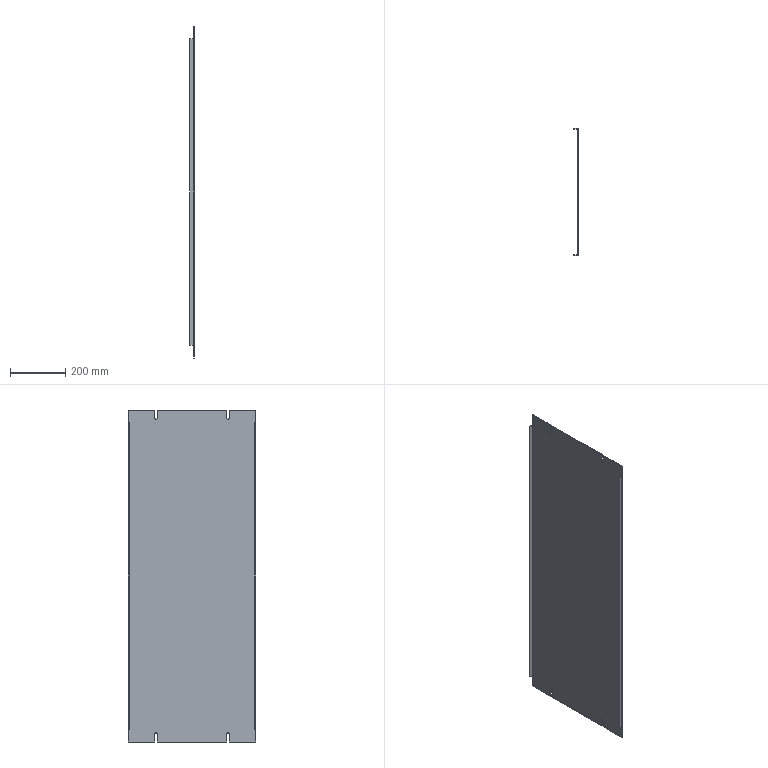Part | STEP file | Electrical board | 1 solid | 48 faces | box 15 x 460 x 1200 mm | volume 1154703 mm3 | plane 38 | cylinder 10 | commonest cylinder face diameters 8 x6 3 x2 7 x2
STEP:
#1=CARTESIAN_POINT('',(2.,-126.,-570.));
#2=VERTEX_POINT('',#1);
#3=CARTESIAN_POINT('',(2.,-130.,-566.));
#4=VERTEX_POINT('',#3);
#5=CARTESIAN_POINT('',(2.,-130.,-570.));
#6=DIRECTION('',(1.,0.,0.));
#7=DIRECTION('',(0.,0.,1.));
#8=AXIS2_PLACEMENT_3D('',#5,#6,#7);
#9=CIRCLE('',#8,4.);
#10=EDGE_CURVE('',#2,#4,#9,.T.);
#11=ORIENTED_EDGE('',*,*,#10,.T.);
#12=CARTESIAN_POINT('',(0.,-130.,-566.));
#13=VERTEX_POINT('',#12);
#14=CARTESIAN_POINT('',(2.,-130.,-566.));
#15=DIRECTION('',(-1.,0.,0.));
#16=VECTOR('',#15,1000.);
#17=LINE('',#14,#16);
#18=EDGE_CURVE('',#4,#13,#17,.T.);
#19=ORIENTED_EDGE('',*,*,#18,.T.);
#20=CARTESIAN_POINT('',(0.,-126.,-570.));
#21=VERTEX_POINT('',#20);
#22=CARTESIAN_POINT('',(0.,-130.,-570.));
#23=DIRECTION('',(1.,0.,0.));
#24=DIRECTION('',(0.,0.,1.));
#25=AXIS2_PLACEMENT_3D('',#22,#23,#24);
#26=CIRCLE('',#25,4.);
#27=EDGE_CURVE('',#21,#13,#26,.T.);
#28=ORIENTED_EDGE('',*,*,#27,.F.);
#29=CARTESIAN_POINT('',(2.,-126.,-570.));
#30=DIRECTION('',(-1.,0.,0.));
#31=VECTOR('',#30,1000.);
#32=LINE('',#29,#31);
#33=EDGE_CURVE('',#2,#21,#32,.T.);
#34=ORIENTED_EDGE('',*,*,#33,.F.);
#35=EDGE_LOOP('',(#11,#19,#28,#34));
#36=FACE_OUTER_BOUND('',#35,.T.);
#37=CARTESIAN_POINT('',(2.,-130.,-570.));
#38=DIRECTION('',(-1.,0.,0.));
#39=DIRECTION('',(0.,0.,1.));
#40=AXIS2_PLACEMENT_3D('',#37,#38,#39);
#41=CYLINDRICAL_SURFACE('',#40,4.);
#42=ADVANCED_FACE('',(#36),#41,.F.);
#43=CARTESIAN_POINT('',(2.,134.,-570.));
#44=VERTEX_POINT('',#43);
#45=CARTESIAN_POINT('',(2.,130.,-566.));
#46=VERTEX_POINT('',#45);
#47=CARTESIAN_POINT('',(2.,130.,-570.));
#48=DIRECTION('',(1.,0.,0.));
#49=DIRECTION('',(0.,0.,1.));
#50=AXIS2_PLACEMENT_3D('',#47,#48,#49);
#51=CIRCLE('',#50,4.);
#52=EDGE_CURVE('',#44,#46,#51,.T.);
#53=ORIENTED_EDGE('',*,*,#52,.T.);
#54=CARTESIAN_POINT('',(0.,130.,-566.));
#55=VERTEX_POINT('',#54);
#56=CARTESIAN_POINT('',(2.,130.,-566.));
#57=DIRECTION('',(-1.,0.,0.));
#58=VECTOR('',#57,1000.);
#59=LINE('',#56,#58);
#60=EDGE_CURVE('',#46,#55,#59,.T.);
#61=ORIENTED_EDGE('',*,*,#60,.T.);
#62=CARTESIAN_POINT('',(0.,134.,-570.));
#63=VERTEX_POINT('',#62);
#64=CARTESIAN_POINT('',(0.,130.,-570.));
#65=DIRECTION('',(1.,0.,0.));
#66=DIRECTION('',(0.,0.,1.));
#67=AXIS2_PLACEMENT_3D('',#64,#65,#66);
#68=CIRCLE('',#67,4.);
#69=EDGE_CURVE('',#63,#55,#68,.T.);
#70=ORIENTED_EDGE('',*,*,#69,.F.);
#71=CARTESIAN_POINT('',(2.,134.,-570.));
#72=DIRECTION('',(-1.,0.,0.));
#73=VECTOR('',#72,1000.);
#74=LINE('',#71,#73);
#75=EDGE_CURVE('',#44,#63,#74,.T.);
#76=ORIENTED_EDGE('',*,*,#75,.F.);
#77=EDGE_LOOP('',(#53,#61,#70,#76));
#78=FACE_OUTER_BOUND('',#77,.T.);
#79=CARTESIAN_POINT('',(2.,130.,-570.));
#80=DIRECTION('',(-1.,0.,0.));
#81=DIRECTION('',(0.,0.,1.));
#82=AXIS2_PLACEMENT_3D('',#79,#80,#81);
#83=CYLINDRICAL_SURFACE('',#82,4.);
#84=ADVANCED_FACE('',(#78),#83,.F.);
#85=CARTESIAN_POINT('',(2.,-225.5,554.));
#86=VERTEX_POINT('',#85);
#87=CARTESIAN_POINT('',(2.,-225.5,555.));
#88=VERTEX_POINT('',#87);
#89=CARTESIAN_POINT('',(2.,-225.5,555.));
#90=DIRECTION('',(0.,0.,1.));
#91=VECTOR('',#90,1000.);
#92=LINE('',#89,#91);
#93=EDGE_CURVE('',#86,#88,#92,.T.);
#94=ORIENTED_EDGE('',*,*,#93,.F.);
#95=CARTESIAN_POINT('',(2.,-226.5,554.));
#96=VERTEX_POINT('',#95);
#97=CARTESIAN_POINT('',(2.,-225.5,554.));
#98=DIRECTION('',(0.,1.,0.));
#99=VECTOR('',#98,1000.);
#100=LINE('',#97,#99);
#101=EDGE_CURVE('',#96,#86,#100,.T.);
#102=ORIENTED_EDGE('',*,*,#101,.F.);
#103=CARTESIAN_POINT('',(2.,-226.5,-554.));
#104=VERTEX_POINT('',#103);
#105=CARTESIAN_POINT('',(2.,-226.5,0.));
#106=DIRECTION('',(0.,0.,1.));
#107=VECTOR('',#106,1000.);
#108=LINE('',#105,#107);
#109=EDGE_CURVE('',#104,#96,#108,.T.);
#110=ORIENTED_EDGE('',*,*,#109,.F.);
#111=CARTESIAN_POINT('',(2.,-225.5,-554.));
#112=VERTEX_POINT('',#111);
#113=CARTESIAN_POINT('',(2.,-226.5,-554.));
#114=DIRECTION('',(0.,-1.,0.));
#115=VECTOR('',#114,1000.);
#116=LINE('',#113,#115);
#117=EDGE_CURVE('',#112,#104,#116,.T.);
#118=ORIENTED_EDGE('',*,*,#117,.F.);
#119=CARTESIAN_POINT('',(2.,-225.5,-555.));
#120=VERTEX_POINT('',#119);
#121=CARTESIAN_POINT('',(2.,-225.5,-554.));
#122=DIRECTION('',(0.,0.,1.));
#123=VECTOR('',#122,1000.);
#124=LINE('',#121,#123);
#125=EDGE_CURVE('',#120,#112,#124,.T.);
#126=ORIENTED_EDGE('',*,*,#125,.F.);
#127=CARTESIAN_POINT('',(2.,-230.,-555.));
#128=VERTEX_POINT('',#127);
#129=CARTESIAN_POINT('',(2.,0.,-555.));
#130=DIRECTION('',(0.,1.,0.));
#131=VECTOR('',#130,1000.);
#132=LINE('',#129,#131);
#133=EDGE_CURVE('',#128,#120,#132,.T.);
#134=ORIENTED_EDGE('',*,*,#133,.F.);
#135=CARTESIAN_POINT('',(2.,-230.,-600.));
#136=VERTEX_POINT('',#135);
#137=CARTESIAN_POINT('',(2.,-230.,0.));
#138=DIRECTION('',(0.,0.,1.));
#139=VECTOR('',#138,1000.);
#140=LINE('',#137,#139);
#141=EDGE_CURVE('',#136,#128,#140,.T.);
#142=ORIENTED_EDGE('',*,*,#141,.F.);
#143=CARTESIAN_POINT('',(2.,-134.,-600.));
#144=VERTEX_POINT('',#143);
#145=CARTESIAN_POINT('',(2.,0.,-600.));
#146=DIRECTION('',(0.,-1.,0.));
#147=VECTOR('',#146,1000.);
#148=LINE('',#145,#147);
#149=EDGE_CURVE('',#144,#136,#148,.T.);
#150=ORIENTED_EDGE('',*,*,#149,.F.);
#151=CARTESIAN_POINT('',(2.,-134.,-570.));
#152=VERTEX_POINT('',#151);
#153=CARTESIAN_POINT('',(2.,-134.,0.));
#154=DIRECTION('',(0.,0.,-1.));
#155=VECTOR('',#154,1000.);
#156=LINE('',#153,#155);
#157=EDGE_CURVE('',#152,#144,#156,.T.);
#158=ORIENTED_EDGE('',*,*,#157,.F.);
#159=CARTESIAN_POINT('',(2.,-130.,-570.));
#160=DIRECTION('',(1.,0.,0.));
#161=DIRECTION('',(0.,0.,1.));
#162=AXIS2_PLACEMENT_3D('',#159,#160,#161);
#163=CIRCLE('',#162,4.);
#164=EDGE_CURVE('',#4,#152,#163,.T.);
#165=ORIENTED_EDGE('',*,*,#164,.F.);
#166=ORIENTED_EDGE('',*,*,#10,.F.);
#167=CARTESIAN_POINT('',(2.,-126.,-600.));
#168=VERTEX_POINT('',#167);
#169=CARTESIAN_POINT('',(2.,-126.,0.));
#170=DIRECTION('',(0.,0.,1.));
#171=VECTOR('',#170,1000.);
#172=LINE('',#169,#171);
#173=EDGE_CURVE('',#168,#2,#172,.T.);
#174=ORIENTED_EDGE('',*,*,#173,.F.);
#175=CARTESIAN_POINT('',(2.,126.,-600.));
#176=VERTEX_POINT('',#175);
#177=CARTESIAN_POINT('',(2.,0.,-600.));
#178=DIRECTION('',(0.,-1.,0.));
#179=VECTOR('',#178,1000.);
#180=LINE('',#177,#179);
#181=EDGE_CURVE('',#176,#168,#180,.T.);
#182=ORIENTED_EDGE('',*,*,#181,.F.);
#183=CARTESIAN_POINT('',(2.,126.,-570.));
#184=VERTEX_POINT('',#183);
#185=CARTESIAN_POINT('',(2.,126.,0.));
#186=DIRECTION('',(0.,0.,-1.));
#187=VECTOR('',#186,1000.);
#188=LINE('',#185,#187);
#189=EDGE_CURVE('',#184,#176,#188,.T.);
#190=ORIENTED_EDGE('',*,*,#189,.F.);
#191=CARTESIAN_POINT('',(2.,130.,-570.));
#192=DIRECTION('',(1.,0.,0.));
#193=DIRECTION('',(0.,0.,1.));
#194=AXIS2_PLACEMENT_3D('',#191,#192,#193);
#195=CIRCLE('',#194,4.);
#196=EDGE_CURVE('',#46,#184,#195,.T.);
#197=ORIENTED_EDGE('',*,*,#196,.F.);
#198=ORIENTED_EDGE('',*,*,#52,.F.);
#199=CARTESIAN_POINT('',(2.,134.,-600.));
#200=VERTEX_POINT('',#199);
#201=CARTESIAN_POINT('',(2.,134.,0.));
#202=DIRECTION('',(0.,0.,1.));
#203=VECTOR('',#202,1000.);
#204=LINE('',#201,#203);
#205=EDGE_CURVE('',#200,#44,#204,.T.);
#206=ORIENTED_EDGE('',*,*,#205,.F.);
#207=CARTESIAN_POINT('',(2.,230.,-600.));
#208=VERTEX_POINT('',#207);
#209=CARTESIAN_POINT('',(2.,0.,-600.));
#210=DIRECTION('',(0.,-1.,0.));
#211=VECTOR('',#210,1000.);
#212=LINE('',#209,#211);
#213=EDGE_CURVE('',#208,#200,#212,.T.);
#214=ORIENTED_EDGE('',*,*,#213,.F.);
#215=CARTESIAN_POINT('',(2.,230.,-555.));
#216=VERTEX_POINT('',#215);
#217=CARTESIAN_POINT('',(2.,230.,0.));
#218=DIRECTION('',(0.,0.,-1.));
#219=VECTOR('',#218,1000.);
#220=LINE('',#217,#219);
#221=EDGE_CURVE('',#216,#208,#220,.T.);
#222=ORIENTED_EDGE('',*,*,#221,.F.);
#223=CARTESIAN_POINT('',(2.,225.5,-555.));
#224=VERTEX_POINT('',#223);
#225=CARTESIAN_POINT('',(2.,0.,-555.));
#226=DIRECTION('',(0.,1.,0.));
#227=VECTOR('',#226,1000.);
#228=LINE('',#225,#227);
#229=EDGE_CURVE('',#224,#216,#228,.T.);
#230=ORIENTED_EDGE('',*,*,#229,.F.);
#231=CARTESIAN_POINT('',(2.,225.5,-554.));
#232=VERTEX_POINT('',#231);
#233=CARTESIAN_POINT('',(2.,225.5,-555.));
#234=DIRECTION('',(0.,0.,-1.));
#235=VECTOR('',#234,1000.);
#236=LINE('',#233,#235);
#237=EDGE_CURVE('',#232,#224,#236,.T.);
#238=ORIENTED_EDGE('',*,*,#237,.F.);
#239=CARTESIAN_POINT('',(2.,226.5,-554.));
#240=VERTEX_POINT('',#239);
#241=CARTESIAN_POINT('',(2.,225.5,-554.));
#242=DIRECTION('',(0.,-1.,0.));
#243=VECTOR('',#242,1000.);
#244=LINE('',#241,#243);
#245=EDGE_CURVE('',#240,#232,#244,.T.);
#246=ORIENTED_EDGE('',*,*,#245,.F.);
#247=CARTESIAN_POINT('',(2.,226.5,554.));
#248=VERTEX_POINT('',#247);
#249=CARTESIAN_POINT('',(2.,226.5,0.));
#250=DIRECTION('',(0.,0.,-1.));
#251=VECTOR('',#250,1000.);
#252=LINE('',#249,#251);
#253=EDGE_CURVE('',#248,#240,#252,.T.);
#254=ORIENTED_EDGE('',*,*,#253,.F.);
#255=CARTESIAN_POINT('',(2.,225.5,554.));
#256=VERTEX_POINT('',#255);
#257=CARTESIAN_POINT('',(2.,226.5,554.));
#258=DIRECTION('',(0.,1.,0.));
#259=VECTOR('',#258,1000.);
#260=LINE('',#257,#259);
#261=EDGE_CURVE('',#256,#248,#260,.T.);
#262=ORIENTED_EDGE('',*,*,#261,.F.);
#263=CARTESIAN_POINT('',(2.,225.5,555.));
#264=VERTEX_POINT('',#263);
#265=CARTESIAN_POINT('',(2.,225.5,554.));
#266=DIRECTION('',(0.,0.,-1.));
#267=VECTOR('',#266,1000.);
#268=LINE('',#265,#267);
#269=EDGE_CURVE('',#264,#256,#268,.T.);
#270=ORIENTED_EDGE('',*,*,#269,.F.);
#271=CARTESIAN_POINT('',(2.,230.,555.));
#272=VERTEX_POINT('',#271);
#273=CARTESIAN_POINT('',(2.,0.,555.));
#274=DIRECTION('',(0.,-1.,0.));
#275=VECTOR('',#274,1000.);
#276=LINE('',#273,#275);
#277=EDGE_CURVE('',#272,#264,#276,.T.);
#278=ORIENTED_EDGE('',*,*,#277,.F.);
#279=CARTESIAN_POINT('',(2.,230.,600.));
#280=VERTEX_POINT('',#279);
#281=CARTESIAN_POINT('',(2.,230.,0.));
#282=DIRECTION('',(0.,0.,-1.));
#283=VECTOR('',#282,1000.);
#284=LINE('',#281,#283);
#285=EDGE_CURVE('',#280,#272,#284,.T.);
#286=ORIENTED_EDGE('',*,*,#285,.F.);
#287=CARTESIAN_POINT('',(2.,134.,600.));
#288=VERTEX_POINT('',#287);
#289=CARTESIAN_POINT('',(2.,0.,600.));
#290=DIRECTION('',(0.,1.,0.));
#291=VECTOR('',#290,1000.);
#292=LINE('',#289,#291);
#293=EDGE_CURVE('',#288,#280,#292,.T.);
#294=ORIENTED_EDGE('',*,*,#293,.F.);
#295=CARTESIAN_POINT('',(2.,134.,570.));
#296=VERTEX_POINT('',#295);
#297=CARTESIAN_POINT('',(2.,134.,0.));
#298=DIRECTION('',(0.,0.,1.));
#299=VECTOR('',#298,1000.);
#300=LINE('',#297,#299);
#301=EDGE_CURVE('',#296,#288,#300,.T.);
#302=ORIENTED_EDGE('',*,*,#301,.F.);
#303=CARTESIAN_POINT('',(2.,126.,570.));
#304=VERTEX_POINT('',#303);
#305=CARTESIAN_POINT('',(2.,130.,570.));
#306=DIRECTION('',(1.,0.,0.));
#307=DIRECTION('',(0.,0.,1.));
#308=AXIS2_PLACEMENT_3D('',#305,#306,#307);
#309=CIRCLE('',#308,4.);
#310=EDGE_CURVE('',#304,#296,#309,.T.);
#311=ORIENTED_EDGE('',*,*,#310,.F.);
#312=CARTESIAN_POINT('',(2.,126.,600.));
#313=VERTEX_POINT('',#312);
#314=CARTESIAN_POINT('',(2.,126.,0.));
#315=DIRECTION('',(0.,0.,-1.));
#316=VECTOR('',#315,1000.);
#317=LINE('',#314,#316);
#318=EDGE_CURVE('',#313,#304,#317,.T.);
#319=ORIENTED_EDGE('',*,*,#318,.F.);
#320=CARTESIAN_POINT('',(2.,-126.,600.));
#321=VERTEX_POINT('',#320);
#322=CARTESIAN_POINT('',(2.,0.,600.));
#323=DIRECTION('',(0.,1.,0.));
#324=VECTOR('',#323,1000.);
#325=LINE('',#322,#324);
#326=EDGE_CURVE('',#321,#313,#325,.T.);
#327=ORIENTED_EDGE('',*,*,#326,.F.);
#328=CARTESIAN_POINT('',(2.,-126.,570.));
#329=VERTEX_POINT('',#328);
#330=CARTESIAN_POINT('',(2.,-126.,0.));
#331=DIRECTION('',(0.,0.,1.));
#332=VECTOR('',#331,1000.);
#333=LINE('',#330,#332);
#334=EDGE_CURVE('',#329,#321,#333,.T.);
#335=ORIENTED_EDGE('',*,*,#334,.F.);
#336=CARTESIAN_POINT('',(2.,-134.,570.));
#337=VERTEX_POINT('',#336);
#338=CARTESIAN_POINT('',(2.,-130.,570.));
#339=DIRECTION('',(1.,0.,0.));
#340=DIRECTION('',(0.,0.,1.));
#341=AXIS2_PLACEMENT_3D('',#338,#339,#340);
#342=CIRCLE('',#341,4.);
#343=EDGE_CURVE('',#337,#329,#342,.T.);
#344=ORIENTED_EDGE('',*,*,#343,.F.);
#345=CARTESIAN_POINT('',(2.,-134.,600.));
#346=VERTEX_POINT('',#345);
#347=CARTESIAN_POINT('',(2.,-134.,0.));
#348=DIRECTION('',(0.,0.,-1.));
#349=VECTOR('',#348,1000.);
#350=LINE('',#347,#349);
#351=EDGE_CURVE('',#346,#337,#350,.T.);
#352=ORIENTED_EDGE('',*,*,#351,.F.);
#353=CARTESIAN_POINT('',(2.,-230.,600.));
#354=VERTEX_POINT('',#353);
#355=CARTESIAN_POINT('',(2.,0.,600.));
#356=DIRECTION('',(0.,1.,0.));
#357=VECTOR('',#356,1000.);
#358=LINE('',#355,#357);
#359=EDGE_CURVE('',#354,#346,#358,.T.);
#360=ORIENTED_EDGE('',*,*,#359,.F.);
#361=CARTESIAN_POINT('',(2.,-230.,555.));
#362=VERTEX_POINT('',#361);
#363=CARTESIAN_POINT('',(2.,-230.,0.));
#364=DIRECTION('',(0.,0.,1.));
#365=VECTOR('',#364,1000.);
#366=LINE('',#363,#365);
#367=EDGE_CURVE('',#362,#354,#366,.T.);
#368=ORIENTED_EDGE('',*,*,#367,.F.);
#369=CARTESIAN_POINT('',(2.,0.,555.));
#370=DIRECTION('',(0.,-1.,0.));
#371=VECTOR('',#370,1000.);
#372=LINE('',#369,#371);
#373=EDGE_CURVE('',#88,#362,#372,.T.);
#374=ORIENTED_EDGE('',*,*,#373,.F.);
#375=EDGE_LOOP('',(#94,#102,#110,#118,#126,#134,#142,#150,#158,#165,#166,#174,#182,#190,#197,#198,#206,#214,#222,#230,#238,#246,#254,#262,#270,#278,#286,#294,#302,#311,#319,#327,#335,#344,#352,#360,#368,#374));
#376=FACE_OUTER_BOUND('',#375,.T.);
#377=CARTESIAN_POINT('',(2.,0.,0.));
#378=DIRECTION('',(-1.,0.,0.));
#379=DIRECTION('',(0.,0.,1.));
#380=AXIS2_PLACEMENT_3D('',#377,#378,#379);
#381=PLANE('',#380);
#382=ADVANCED_FACE('',(#376),#381,.F.);
#383=CARTESIAN_POINT('',(0.,-225.5,555.));
#384=VERTEX_POINT('',#383);
#385=CARTESIAN_POINT('',(0.,-230.,555.));
#386=VERTEX_POINT('',#385);
#387=CARTESIAN_POINT('',(0.,-232.,555.));
#388=DIRECTION('',(0.,-1.,0.));
#389=VECTOR('',#388,1000.);
#390=LINE('',#387,#389);
#391=EDGE_CURVE('',#384,#386,#390,.T.);
#392=ORIENTED_EDGE('',*,*,#391,.F.);
#393=CARTESIAN_POINT('',(2.,-225.5,555.));
#394=DIRECTION('',(-1.,0.,0.));
#395=VECTOR('',#394,1000.);
#396=LINE('',#393,#395);
#397=EDGE_CURVE('',#88,#384,#396,.T.);
#398=ORIENTED_EDGE('',*,*,#397,.F.);
#399=ORIENTED_EDGE('',*,*,#373,.T.);
#400=CARTESIAN_POINT('',(2.,-230.,555.));
#401=DIRECTION('',(1.,0.,0.));
#402=VECTOR('',#401,1000.);
#403=LINE('',#400,#402);
#404=EDGE_CURVE('',#386,#362,#403,.T.);
#405=ORIENTED_EDGE('',*,*,#404,.F.);
#406=EDGE_LOOP('',(#392,#398,#399,#405));
#407=FACE_OUTER_BOUND('',#406,.T.);
#408=CARTESIAN_POINT('',(2.,-232.,555.));
#409=DIRECTION('',(0.,0.,1.));
#410=DIRECTION('',(1.,0.,0.));
#411=AXIS2_PLACEMENT_3D('',#408,#409,#410);
#412=PLANE('',#411);
#413=ADVANCED_FACE('',(#407),#412,.F.);
#414=CARTESIAN_POINT('',(-1.5,-230.,554.));
#415=VERTEX_POINT('',#414);
#416=CARTESIAN_POINT('',(-1.5,-230.,-554.));
#417=VERTEX_POINT('',#416);
#418=CARTESIAN_POINT('',(-1.5,-230.,554.));
#419=DIRECTION('',(0.,0.,-1.));
#420=VECTOR('',#419,1000.);
#421=LINE('',#418,#420);
#422=EDGE_CURVE('',#415,#417,#421,.T.);
#423=ORIENTED_EDGE('',*,*,#422,.T.);
#424=CARTESIAN_POINT('',(-1.5,-226.5,-554.));
#425=DIRECTION('',(0.,0.,1.));
#426=DIRECTION('',(1.,0.,0.));
#427=AXIS2_PLACEMENT_3D('',#424,#425,#426);
#428=CIRCLE('',#427,3.5);
#429=EDGE_CURVE('',#417,#104,#428,.T.);
#430=ORIENTED_EDGE('',*,*,#429,.T.);
#431=ORIENTED_EDGE('',*,*,#109,.T.);
#432=CARTESIAN_POINT('',(-1.5,-226.5,554.));
#433=DIRECTION('',(0.,0.,-1.));
#434=DIRECTION('',(1.,0.,0.));
#435=AXIS2_PLACEMENT_3D('',#432,#433,#434);
#436=CIRCLE('',#435,3.5);
#437=EDGE_CURVE('',#96,#415,#436,.T.);
#438=ORIENTED_EDGE('',*,*,#437,.T.);
#439=EDGE_LOOP('',(#423,#430,#431,#438));
#440=FACE_OUTER_BOUND('',#439,.T.);
#441=CARTESIAN_POINT('',(-1.5,-226.5,554.));
#442=DIRECTION('',(0.,0.,1.));
#443=DIRECTION('',(1.,0.,0.));
#444=AXIS2_PLACEMENT_3D('',#441,#442,#443);
#445=CYLINDRICAL_SURFACE('',#444,3.5);
#446=ADVANCED_FACE('',(#440),#445,.T.);
#447=CARTESIAN_POINT('',(0.,-225.5,-555.));
#448=VERTEX_POINT('',#447);
#449=CARTESIAN_POINT('',(0.,-230.,-555.));
#450=VERTEX_POINT('',#449);
#451=CARTESIAN_POINT('',(0.,-232.,-555.));
#452=DIRECTION('',(0.,-1.,0.));
#453=VECTOR('',#452,1000.);
#454=LINE('',#451,#453);
#455=EDGE_CURVE('',#448,#450,#454,.T.);
#456=ORIENTED_EDGE('',*,*,#455,.T.);
#457=CARTESIAN_POINT('',(2.,-230.,-555.));
#458=DIRECTION('',(1.,0.,0.));
#459=VECTOR('',#458,1000.);
#460=LINE('',#457,#459);
#461=EDGE_CURVE('',#450,#128,#460,.T.);
#462=ORIENTED_EDGE('',*,*,#461,.T.);
#463=ORIENTED_EDGE('',*,*,#133,.T.);
#464=CARTESIAN_POINT('',(2.,-225.5,-555.));
#465=DIRECTION('',(-1.,0.,0.));
#466=VECTOR('',#465,1000.);
#467=LINE('',#464,#466);
#468=EDGE_CURVE('',#120,#448,#467,.T.);
#469=ORIENTED_EDGE('',*,*,#468,.T.);
#470=EDGE_LOOP('',(#456,#462,#463,#469));
#471=FACE_OUTER_BOUND('',#470,.T.);
#472=CARTESIAN_POINT('',(2.,-232.,-555.));
#473=DIRECTION('',(0.,0.,1.));
#474=DIRECTION('',(1.,0.,0.));
#475=AXIS2_PLACEMENT_3D('',#472,#473,#474);
#476=PLANE('',#475);
#477=ADVANCED_FACE('',(#471),#476,.T.);
#478=CARTESIAN_POINT('',(0.,-230.,-600.));
#479=VERTEX_POINT('',#478);
#480=CARTESIAN_POINT('',(0.,-230.,600.));
#481=DIRECTION('',(0.,0.,1.));
#482=VECTOR('',#481,1000.);
#483=LINE('',#480,#482);
#484=EDGE_CURVE('',#479,#450,#483,.T.);
#485=ORIENTED_EDGE('',*,*,#484,.F.);
#486=CARTESIAN_POINT('',(2.,-230.,-600.));
#487=DIRECTION('',(-1.,0.,0.));
#488=VECTOR('',#487,1000.);
#489=LINE('',#486,#488);
#490=EDGE_CURVE('',#136,#479,#489,.T.);
#491=ORIENTED_EDGE('',*,*,#490,.F.);
#492=ORIENTED_EDGE('',*,*,#141,.T.);
#493=ORIENTED_EDGE('',*,*,#461,.F.);
#494=EDGE_LOOP('',(#485,#491,#492,#493));
#495=FACE_OUTER_BOUND('',#494,.T.);
#496=CARTESIAN_POINT('',(2.,-230.,600.));
#497=DIRECTION('',(0.,1.,0.));
#498=DIRECTION('',(0.,0.,1.));
#499=AXIS2_PLACEMENT_3D('',#496,#497,#498);
#500=PLANE('',#499);
#501=ADVANCED_FACE('',(#495),#500,.F.);
#502=CARTESIAN_POINT('',(0.,-134.,-600.));
#503=VERTEX_POINT('',#502);
#504=CARTESIAN_POINT('',(0.,-230.,-600.));
#505=DIRECTION('',(0.,-1.,0.));
#506=VECTOR('',#505,1000.);
#507=LINE('',#504,#506);
#508=EDGE_CURVE('',#503,#479,#507,.T.);
#509=ORIENTED_EDGE('',*,*,#508,.F.);
#510=CARTESIAN_POINT('',(2.,-134.,-600.));
#511=DIRECTION('',(-1.,0.,0.));
#512=VECTOR('',#511,1000.);
#513=LINE('',#510,#512);
#514=EDGE_CURVE('',#144,#503,#513,.T.);
#515=ORIENTED_EDGE('',*,*,#514,.F.);
#516=ORIENTED_EDGE('',*,*,#149,.T.);
#517=ORIENTED_EDGE('',*,*,#490,.T.);
#518=EDGE_LOOP('',(#509,#515,#516,#517));
#519=FACE_OUTER_BOUND('',#518,.T.);
#520=CARTESIAN_POINT('',(2.,-230.,-600.));
#521=DIRECTION('',(0.,0.,1.));
#522=DIRECTION('',(1.,0.,0.));
#523=AXIS2_PLACEMENT_3D('',#520,#521,#522);
#524=PLANE('',#523);
#525=ADVANCED_FACE('',(#519),#524,.F.);
#526=CARTESIAN_POINT('',(0.,-134.,-570.));
#527=VERTEX_POINT('',#526);
#528=CARTESIAN_POINT('',(0.,-134.,-630.));
#529=DIRECTION('',(0.,0.,-1.));
#530=VECTOR('',#529,1000.);
#531=LINE('',#528,#530);
#532=EDGE_CURVE('',#527,#503,#531,.T.);
#533=ORIENTED_EDGE('',*,*,#532,.F.);
#534=CARTESIAN_POINT('',(2.,-134.,-570.));
#535=DIRECTION('',(-1.,0.,0.));
#536=VECTOR('',#535,1000.);
#537=LINE('',#534,#536);
#538=EDGE_CURVE('',#152,#527,#537,.T.);
#539=ORIENTED_EDGE('',*,*,#538,.F.);
#540=ORIENTED_EDGE('',*,*,#157,.T.);
#541=ORIENTED_EDGE('',*,*,#514,.T.);
#542=EDGE_LOOP('',(#533,#539,#540,#541));
#543=FACE_OUTER_BOUND('',#542,.T.);
#544=CARTESIAN_POINT('',(2.,-134.,-630.));
#545=DIRECTION('',(0.,-1.,0.));
#546=DIRECTION('',(0.,0.,-1.));
#547=AXIS2_PLACEMENT_3D('',#544,#545,#546);
#548=PLANE('',#547);
#549=ADVANCED_FACE('',(#543),#548,.F.);
#550=ORIENTED_EDGE('',*,*,#18,.F.);
#551=ORIENTED_EDGE('',*,*,#164,.T.);
#552=ORIENTED_EDGE('',*,*,#538,.T.);
#553=CARTESIAN_POINT('',(0.,-130.,-570.));
#554=DIRECTION('',(1.,0.,0.));
#555=DIRECTION('',(0.,0.,1.));
#556=AXIS2_PLACEMENT_3D('',#553,#554,#555);
#557=CIRCLE('',#556,4.);
#558=EDGE_CURVE('',#13,#527,#557,.T.);
#559=ORIENTED_EDGE('',*,*,#558,.F.);
#560=EDGE_LOOP('',(#550,#551,#552,#559));
#561=FACE_OUTER_BOUND('',#560,.T.);
#562=CARTESIAN_POINT('',(2.,-130.,-570.));
#563=DIRECTION('',(-1.,0.,0.));
#564=DIRECTION('',(0.,0.,1.));
#565=AXIS2_PLACEMENT_3D('',#562,#563,#564);
#566=CYLINDRICAL_SURFACE('',#565,4.);
#567=ADVANCED_FACE('',(#561),#566,.F.);
#568=CARTESIAN_POINT('',(0.,-126.,-600.));
#569=VERTEX_POINT('',#568);
#570=CARTESIAN_POINT('',(0.,-126.,-630.));
#571=DIRECTION('',(0.,0.,1.));
#572=VECTOR('',#571,1000.);
#573=LINE('',#570,#572);
#574=EDGE_CURVE('',#569,#21,#573,.T.);
#575=ORIENTED_EDGE('',*,*,#574,.F.);
#576=CARTESIAN_POINT('',(2.,-126.,-600.));
#577=DIRECTION('',(-1.,0.,0.));
#578=VECTOR('',#577,1000.);
#579=LINE('',#576,#578);
#580=EDGE_CURVE('',#168,#569,#579,.T.);
#581=ORIENTED_EDGE('',*,*,#580,.F.);
#582=ORIENTED_EDGE('',*,*,#173,.T.);
#583=ORIENTED_EDGE('',*,*,#33,.T.);
#584=EDGE_LOOP('',(#575,#581,#582,#583));
#585=FACE_OUTER_BOUND('',#584,.T.);
#586=CARTESIAN_POINT('',(2.,-126.,-630.));
#587=DIRECTION('',(0.,1.,0.));
#588=DIRECTION('',(0.,0.,1.));
#589=AXIS2_PLACEMENT_3D('',#586,#587,#588);
#590=PLANE('',#589);
#591=ADVANCED_FACE('',(#585),#590,.F.);
#592=CARTESIAN_POINT('',(0.,126.,-600.));
#593=VERTEX_POINT('',#592);
#594=CARTESIAN_POINT('',(0.,-230.,-600.));
#595=DIRECTION('',(0.,-1.,0.));
#596=VECTOR('',#595,1000.);
#597=LINE('',#594,#596);
#598=EDGE_CURVE('',#593,#569,#597,.T.);
#599=ORIENTED_EDGE('',*,*,#598,.F.);
#600=CARTESIAN_POINT('',(2.,126.,-600.));
#601=DIRECTION('',(-1.,0.,0.));
#602=VECTOR('',#601,1000.);
#603=LINE('',#600,#602);
#604=EDGE_CURVE('',#176,#593,#603,.T.);
#605=ORIENTED_EDGE('',*,*,#604,.F.);
#606=ORIENTED_EDGE('',*,*,#181,.T.);
#607=ORIENTED_EDGE('',*,*,#580,.T.);
#608=EDGE_LOOP('',(#599,#605,#606,#607));
#609=FACE_OUTER_BOUND('',#608,.T.);
#610=CARTESIAN_POINT('',(2.,-230.,-600.));
#611=DIRECTION('',(0.,0.,1.));
#612=DIRECTION('',(1.,0.,0.));
#613=AXIS2_PLACEMENT_3D('',#610,#611,#612);
#614=PLANE('',#613);
#615=ADVANCED_FACE('',(#609),#614,.F.);
#616=CARTESIAN_POINT('',(0.,126.,-570.));
#617=VERTEX_POINT('',#616);
#618=CARTESIAN_POINT('',(0.,126.,-630.));
#619=DIRECTION('',(0.,0.,-1.));
#620=VECTOR('',#619,1000.);
#621=LINE('',#618,#620);
#622=EDGE_CURVE('',#617,#593,#621,.T.);
#623=ORIENTED_EDGE('',*,*,#622,.F.);
#624=CARTESIAN_POINT('',(2.,126.,-570.));
#625=DIRECTION('',(-1.,0.,0.));
#626=VECTOR('',#625,1000.);
#627=LINE('',#624,#626);
#628=EDGE_CURVE('',#184,#617,#627,.T.);
#629=ORIENTED_EDGE('',*,*,#628,.F.);
#630=ORIENTED_EDGE('',*,*,#189,.T.);
#631=ORIENTED_EDGE('',*,*,#604,.T.);
#632=EDGE_LOOP('',(#623,#629,#630,#631));
#633=FACE_OUTER_BOUND('',#632,.T.);
#634=CARTESIAN_POINT('',(2.,126.,-630.));
#635=DIRECTION('',(0.,-1.,0.));
#636=DIRECTION('',(0.,0.,-1.));
#637=AXIS2_PLACEMENT_3D('',#634,#635,#636);
#638=PLANE('',#637);
#639=ADVANCED_FACE('',(#633),#638,.F.);
#640=ORIENTED_EDGE('',*,*,#60,.F.);
#641=ORIENTED_EDGE('',*,*,#196,.T.);
#642=ORIENTED_EDGE('',*,*,#628,.T.);
#643=CARTESIAN_POINT('',(0.,130.,-570.));
#644=DIRECTION('',(1.,0.,0.));
#645=DIRECTION('',(0.,0.,1.));
#646=AXIS2_PLACEMENT_3D('',#643,#644,#645);
#647=CIRCLE('',#646,4.);
#648=EDGE_CURVE('',#55,#617,#647,.T.);
#649=ORIENTED_EDGE('',*,*,#648,.F.);
#650=EDGE_LOOP('',(#640,#641,#642,#649));
#651=FACE_OUTER_BOUND('',#650,.T.);
#652=CARTESIAN_POINT('',(2.,130.,-570.));
#653=DIRECTION('',(-1.,0.,0.));
#654=DIRECTION('',(0.,0.,1.));
#655=AXIS2_PLACEMENT_3D('',#652,#653,#654);
#656=CYLINDRICAL_SURFACE('',#655,4.);
#657=ADVANCED_FACE('',(#651),#656,.F.);
#658=CARTESIAN_POINT('',(0.,134.,-600.));
#659=VERTEX_POINT('',#658);
#660=CARTESIAN_POINT('',(0.,134.,-630.));
#661=DIRECTION('',(0.,0.,1.));
#662=VECTOR('',#661,1000.);
#663=LINE('',#660,#662);
#664=EDGE_CURVE('',#659,#63,#663,.T.);
#665=ORIENTED_EDGE('',*,*,#664,.F.);
#666=CARTESIAN_POINT('',(2.,134.,-600.));
#667=DIRECTION('',(-1.,0.,0.));
#668=VECTOR('',#667,1000.);
#669=LINE('',#666,#668);
#670=EDGE_CURVE('',#200,#659,#669,.T.);
#671=ORIENTED_EDGE('',*,*,#670,.F.);
#672=ORIENTED_EDGE('',*,*,#205,.T.);
#673=ORIENTED_EDGE('',*,*,#75,.T.);
#674=EDGE_LOOP('',(#665,#671,#672,#673));
#675=FACE_OUTER_BOUND('',#674,.T.);
#676=CARTESIAN_POINT('',(2.,134.,-630.));
#677=DIRECTION('',(0.,1.,0.));
#678=DIRECTION('',(0.,0.,1.));
#679=AXIS2_PLACEMENT_3D('',#676,#677,#678);
#680=PLANE('',#679);
#681=ADVANCED_FACE('',(#675),#680,.F.);
#682=CARTESIAN_POINT('',(0.,230.,-600.));
#683=VERTEX_POINT('',#682);
#684=CARTESIAN_POINT('',(0.,-230.,-600.));
#685=DIRECTION('',(0.,-1.,0.));
#686=VECTOR('',#685,1000.);
#687=LINE('',#684,#686);
#688=EDGE_CURVE('',#683,#659,#687,.T.);
#689=ORIENTED_EDGE('',*,*,#688,.F.);
#690=CARTESIAN_POINT('',(2.,230.,-600.));
#691=DIRECTION('',(-1.,0.,0.));
#692=VECTOR('',#691,1000.);
#693=LINE('',#690,#692);
#694=EDGE_CURVE('',#208,#683,#693,.T.);
#695=ORIENTED_EDGE('',*,*,#694,.F.);
#696=ORIENTED_EDGE('',*,*,#213,.T.);
#697=ORIENTED_EDGE('',*,*,#670,.T.);
#698=EDGE_LOOP('',(#689,#695,#696,#697));
#699=FACE_OUTER_BOUND('',#698,.T.);
#700=CARTESIAN_POINT('',(2.,-230.,-600.));
#701=DIRECTION('',(0.,0.,1.));
#702=DIRECTION('',(1.,0.,0.));
#703=AXIS2_PLACEMENT_3D('',#700,#701,#702);
#704=PLANE('',#703);
#705=ADVANCED_FACE('',(#699),#704,.F.);
#706=CARTESIAN_POINT('',(0.,230.,-555.));
#707=VERTEX_POINT('',#706);
#708=CARTESIAN_POINT('',(0.,230.,600.));
#709=DIRECTION('',(0.,0.,-1.));
#710=VECTOR('',#709,1000.);
#711=LINE('',#708,#710);
#712=EDGE_CURVE('',#707,#683,#711,.T.);
#713=ORIENTED_EDGE('',*,*,#712,.F.);
#714=CARTESIAN_POINT('',(2.,230.,-555.));
#715=DIRECTION('',(-1.,0.,0.));
#716=VECTOR('',#715,1000.);
#717=LINE('',#714,#716);
#718=EDGE_CURVE('',#216,#707,#717,.T.);
#719=ORIENTED_EDGE('',*,*,#718,.F.);
#720=ORIENTED_EDGE('',*,*,#221,.T.);
#721=ORIENTED_EDGE('',*,*,#694,.T.);
#722=EDGE_LOOP('',(#713,#719,#720,#721));
#723=FACE_OUTER_BOUND('',#722,.T.);
#724=CARTESIAN_POINT('',(2.,230.,600.));
#725=DIRECTION('',(0.,-1.,0.));
#726=DIRECTION('',(0.,0.,-1.));
#727=AXIS2_PLACEMENT_3D('',#724,#725,#726);
#728=PLANE('',#727);
#729=ADVANCED_FACE('',(#723),#728,.F.);
#730=CARTESIAN_POINT('',(0.,225.5,-555.));
#731=VERTEX_POINT('',#730);
#732=CARTESIAN_POINT('',(0.,232.,-555.));
#733=DIRECTION('',(0.,1.,0.));
#734=VECTOR('',#733,1000.);
#735=LINE('',#732,#734);
#736=EDGE_CURVE('',#731,#707,#735,.T.);
#737=ORIENTED_EDGE('',*,*,#736,.F.);
#738=CARTESIAN_POINT('',(2.,225.5,-555.));
#739=DIRECTION('',(-1.,0.,0.));
#740=VECTOR('',#739,1000.);
#741=LINE('',#738,#740);
#742=EDGE_CURVE('',#224,#731,#741,.T.);
#743=ORIENTED_EDGE('',*,*,#742,.F.);
#744=ORIENTED_EDGE('',*,*,#229,.T.);
#745=ORIENTED_EDGE('',*,*,#718,.T.);
#746=EDGE_LOOP('',(#737,#743,#744,#745));
#747=FACE_OUTER_BOUND('',#746,.T.);
#748=CARTESIAN_POINT('',(2.,232.,-555.));
#749=DIRECTION('',(0.,0.,-1.));
#750=DIRECTION('',(-1.,0.,0.));
#751=AXIS2_PLACEMENT_3D('',#748,#749,#750);
#752=PLANE('',#751);
#753=ADVANCED_FACE('',(#747),#752,.F.);
#754=CARTESIAN_POINT('',(-1.5,230.,-554.));
#755=VERTEX_POINT('',#754);
#756=CARTESIAN_POINT('',(-1.5,230.,554.));
#757=VERTEX_POINT('',#756);
#758=CARTESIAN_POINT('',(-1.5,230.,-554.));
#759=DIRECTION('',(0.,0.,1.));
#760=VECTOR('',#759,1000.);
#761=LINE('',#758,#760);
#762=EDGE_CURVE('',#755,#757,#761,.T.);
#763=ORIENTED_EDGE('',*,*,#762,.T.);
#764=CARTESIAN_POINT('',(-1.5,226.5,554.));
#765=DIRECTION('',(0.,0.,-1.));
#766=DIRECTION('',(-1.,0.,0.));
#767=AXIS2_PLACEMENT_3D('',#764,#765,#766);
#768=CIRCLE('',#767,3.5);
#769=EDGE_CURVE('',#757,#248,#768,.T.);
#770=ORIENTED_EDGE('',*,*,#769,.T.);
#771=ORIENTED_EDGE('',*,*,#253,.T.);
#772=CARTESIAN_POINT('',(-1.5,226.5,-554.));
#773=DIRECTION('',(0.,0.,1.));
#774=DIRECTION('',(-1.,0.,0.));
#775=AXIS2_PLACEMENT_3D('',#772,#773,#774);
#776=CIRCLE('',#775,3.5);
#777=EDGE_CURVE('',#240,#755,#776,.T.);
#778=ORIENTED_EDGE('',*,*,#777,.T.);
#779=EDGE_LOOP('',(#763,#770,#771,#778));
#780=FACE_OUTER_BOUND('',#779,.T.);
#781=CARTESIAN_POINT('',(-1.5,226.5,-554.));
#782=DIRECTION('',(0.,0.,-1.));
#783=DIRECTION('',(-1.,0.,0.));
#784=AXIS2_PLACEMENT_3D('',#781,#782,#783);
#785=CYLINDRICAL_SURFACE('',#784,3.5);
#786=ADVANCED_FACE('',(#780),#785,.T.);
#787=CARTESIAN_POINT('',(0.,225.5,555.));
#788=VERTEX_POINT('',#787);
#789=CARTESIAN_POINT('',(0.,230.,555.));
#790=VERTEX_POINT('',#789);
#791=CARTESIAN_POINT('',(0.,232.,555.));
#792=DIRECTION('',(0.,1.,0.));
#793=VECTOR('',#792,1000.);
#794=LINE('',#791,#793);
#795=EDGE_CURVE('',#788,#790,#794,.T.);
#796=ORIENTED_EDGE('',*,*,#795,.T.);
#797=CARTESIAN_POINT('',(2.,230.,555.));
#798=DIRECTION('',(1.,0.,0.));
#799=VECTOR('',#798,1000.);
#800=LINE('',#797,#799);
#801=EDGE_CURVE('',#790,#272,#800,.T.);
#802=ORIENTED_EDGE('',*,*,#801,.T.);
#803=ORIENTED_EDGE('',*,*,#277,.T.);
#804=CARTESIAN_POINT('',(2.,225.5,555.));
#805=DIRECTION('',(-1.,0.,0.));
#806=VECTOR('',#805,1000.);
#807=LINE('',#804,#806);
#808=EDGE_CURVE('',#264,#788,#807,.T.);
#809=ORIENTED_EDGE('',*,*,#808,.T.);
#810=EDGE_LOOP('',(#796,#802,#803,#809));
#811=FACE_OUTER_BOUND('',#810,.T.);
#812=CARTESIAN_POINT('',(2.,232.,555.));
#813=DIRECTION('',(0.,0.,-1.));
#814=DIRECTION('',(-1.,0.,0.));
#815=AXIS2_PLACEMENT_3D('',#812,#813,#814);
#816=PLANE('',#815);
#817=ADVANCED_FACE('',(#811),#816,.T.);
#818=CARTESIAN_POINT('',(0.,230.,600.));
#819=VERTEX_POINT('',#818);
#820=CARTESIAN_POINT('',(0.,230.,600.));
#821=DIRECTION('',(0.,0.,-1.));
#822=VECTOR('',#821,1000.);
#823=LINE('',#820,#822);
#824=EDGE_CURVE('',#819,#790,#823,.T.);
#825=ORIENTED_EDGE('',*,*,#824,.F.);
#826=CARTESIAN_POINT('',(2.,230.,600.));
#827=DIRECTION('',(-1.,0.,0.));
#828=VECTOR('',#827,1000.);
#829=LINE('',#826,#828);
#830=EDGE_CURVE('',#280,#819,#829,.T.);
#831=ORIENTED_EDGE('',*,*,#830,.F.);
#832=ORIENTED_EDGE('',*,*,#285,.T.);
#833=ORIENTED_EDGE('',*,*,#801,.F.);
#834=EDGE_LOOP('',(#825,#831,#832,#833));
#835=FACE_OUTER_BOUND('',#834,.T.);
#836=CARTESIAN_POINT('',(2.,230.,600.));
#837=DIRECTION('',(0.,-1.,0.));
#838=DIRECTION('',(0.,0.,-1.));
#839=AXIS2_PLACEMENT_3D('',#836,#837,#838);
#840=PLANE('',#839);
#841=ADVANCED_FACE('',(#835),#840,.F.);
#842=CARTESIAN_POINT('',(0.,134.,600.));
#843=VERTEX_POINT('',#842);
#844=CARTESIAN_POINT('',(0.,-230.,600.));
#845=DIRECTION('',(0.,1.,0.));
#846=VECTOR('',#845,1000.);
#847=LINE('',#844,#846);
#848=EDGE_CURVE('',#843,#819,#847,.T.);
#849=ORIENTED_EDGE('',*,*,#848,.F.);
#850=CARTESIAN_POINT('',(2.,134.,600.));
#851=DIRECTION('',(-1.,0.,0.));
#852=VECTOR('',#851,1000.);
#853=LINE('',#850,#852);
#854=EDGE_CURVE('',#288,#843,#853,.T.);
#855=ORIENTED_EDGE('',*,*,#854,.F.);
#856=ORIENTED_EDGE('',*,*,#293,.T.);
#857=ORIENTED_EDGE('',*,*,#830,.T.);
#858=EDGE_LOOP('',(#849,#855,#856,#857));
#859=FACE_OUTER_BOUND('',#858,.T.);
#860=CARTESIAN_POINT('',(2.,-230.,600.));
#861=DIRECTION('',(0.,0.,-1.));
#862=DIRECTION('',(-1.,0.,0.));
#863=AXIS2_PLACEMENT_3D('',#860,#861,#862);
#864=PLANE('',#863);
#865=ADVANCED_FACE('',(#859),#864,.F.);
#866=CARTESIAN_POINT('',(0.,134.,570.));
#867=VERTEX_POINT('',#866);
#868=CARTESIAN_POINT('',(2.,134.,570.));
#869=DIRECTION('',(1.,0.,0.));
#870=VECTOR('',#869,1000.);
#871=LINE('',#868,#870);
#872=EDGE_CURVE('',#867,#296,#871,.T.);
#873=ORIENTED_EDGE('',*,*,#872,.T.);
#874=ORIENTED_EDGE('',*,*,#301,.T.);
#875=ORIENTED_EDGE('',*,*,#854,.T.);
#876=CARTESIAN_POINT('',(0.,134.,630.));
#877=DIRECTION('',(0.,0.,-1.));
#878=VECTOR('',#877,1000.);
#879=LINE('',#876,#878);
#880=EDGE_CURVE('',#843,#867,#879,.T.);
#881=ORIENTED_EDGE('',*,*,#880,.T.);
#882=EDGE_LOOP('',(#873,#874,#875,#881));
#883=FACE_OUTER_BOUND('',#882,.T.);
#884=CARTESIAN_POINT('',(2.,134.,630.));
#885=DIRECTION('',(0.,-1.,0.));
#886=DIRECTION('',(0.,0.,-1.));
#887=AXIS2_PLACEMENT_3D('',#884,#885,#886);
#888=PLANE('',#887);
#889=ADVANCED_FACE('',(#883),#888,.T.);
#890=CARTESIAN_POINT('',(0.,126.,570.));
#891=VERTEX_POINT('',#890);
#892=CARTESIAN_POINT('',(0.,130.,570.));
#893=DIRECTION('',(1.,0.,0.));
#894=DIRECTION('',(0.,0.,1.));
#895=AXIS2_PLACEMENT_3D('',#892,#893,#894);
#896=CIRCLE('',#895,4.);
#897=EDGE_CURVE('',#891,#867,#896,.T.);
#898=ORIENTED_EDGE('',*,*,#897,.F.);
#899=CARTESIAN_POINT('',(2.,126.,570.));
#900=DIRECTION('',(-1.,0.,0.));
#901=VECTOR('',#900,1000.);
#902=LINE('',#899,#901);
#903=EDGE_CURVE('',#304,#891,#902,.T.);
#904=ORIENTED_EDGE('',*,*,#903,.F.);
#905=ORIENTED_EDGE('',*,*,#310,.T.);
#906=ORIENTED_EDGE('',*,*,#872,.F.);
#907=EDGE_LOOP('',(#898,#904,#905,#906));
#908=FACE_OUTER_BOUND('',#907,.T.);
#909=CARTESIAN_POINT('',(2.,130.,570.));
#910=DIRECTION('',(-1.,0.,0.));
#911=DIRECTION('',(0.,0.,1.));
#912=AXIS2_PLACEMENT_3D('',#909,#910,#911);
#913=CYLINDRICAL_SURFACE('',#912,4.);
#914=ADVANCED_FACE('',(#908),#913,.F.);
#915=CARTESIAN_POINT('',(0.,126.,600.));
#916=VERTEX_POINT('',#915);
#917=CARTESIAN_POINT('',(2.,126.,600.));
#918=DIRECTION('',(1.,0.,0.));
#919=VECTOR('',#918,1000.);
#920=LINE('',#917,#919);
#921=EDGE_CURVE('',#916,#313,#920,.T.);
#922=ORIENTED_EDGE('',*,*,#921,.T.);
#923=ORIENTED_EDGE('',*,*,#318,.T.);
#924=ORIENTED_EDGE('',*,*,#903,.T.);
#925=CARTESIAN_POINT('',(0.,126.,630.));
#926=DIRECTION('',(0.,0.,1.));
#927=VECTOR('',#926,1000.);
#928=LINE('',#925,#927);
#929=EDGE_CURVE('',#891,#916,#928,.T.);
#930=ORIENTED_EDGE('',*,*,#929,.T.);
#931=EDGE_LOOP('',(#922,#923,#924,#930));
#932=FACE_OUTER_BOUND('',#931,.T.);
#933=CARTESIAN_POINT('',(2.,126.,630.));
#934=DIRECTION('',(0.,1.,0.));
#935=DIRECTION('',(0.,0.,1.));
#936=AXIS2_PLACEMENT_3D('',#933,#934,#935);
#937=PLANE('',#936);
#938=ADVANCED_FACE('',(#932),#937,.T.);
#939=CARTESIAN_POINT('',(0.,-126.,600.));
#940=VERTEX_POINT('',#939);
#941=CARTESIAN_POINT('',(0.,-230.,600.));
#942=DIRECTION('',(0.,1.,0.));
#943=VECTOR('',#942,1000.);
#944=LINE('',#941,#943);
#945=EDGE_CURVE('',#940,#916,#944,.T.);
#946=ORIENTED_EDGE('',*,*,#945,.F.);
#947=CARTESIAN_POINT('',(2.,-126.,600.));
#948=DIRECTION('',(-1.,0.,0.));
#949=VECTOR('',#948,1000.);
#950=LINE('',#947,#949);
#951=EDGE_CURVE('',#321,#940,#950,.T.);
#952=ORIENTED_EDGE('',*,*,#951,.F.);
#953=ORIENTED_EDGE('',*,*,#326,.T.);
#954=ORIENTED_EDGE('',*,*,#921,.F.);
#955=EDGE_LOOP('',(#946,#952,#953,#954));
#956=FACE_OUTER_BOUND('',#955,.T.);
#957=CARTESIAN_POINT('',(2.,-230.,600.));
#958=DIRECTION('',(0.,0.,-1.));
#959=DIRECTION('',(-1.,0.,0.));
#960=AXIS2_PLACEMENT_3D('',#957,#958,#959);
#961=PLANE('',#960);
#962=ADVANCED_FACE('',(#956),#961,.F.);
#963=CARTESIAN_POINT('',(0.,-126.,570.));
#964=VERTEX_POINT('',#963);
#965=CARTESIAN_POINT('',(2.,-126.,570.));
#966=DIRECTION('',(1.,0.,0.));
#967=VECTOR('',#966,1000.);
#968=LINE('',#965,#967);
#969=EDGE_CURVE('',#964,#329,#968,.T.);
#970=ORIENTED_EDGE('',*,*,#969,.T.);
#971=ORIENTED_EDGE('',*,*,#334,.T.);
#972=ORIENTED_EDGE('',*,*,#951,.T.);
#973=CARTESIAN_POINT('',(0.,-126.,630.));
#974=DIRECTION('',(0.,0.,-1.));
#975=VECTOR('',#974,1000.);
#976=LINE('',#973,#975);
#977=EDGE_CURVE('',#940,#964,#976,.T.);
#978=ORIENTED_EDGE('',*,*,#977,.T.);
#979=EDGE_LOOP('',(#970,#971,#972,#978));
#980=FACE_OUTER_BOUND('',#979,.T.);
#981=CARTESIAN_POINT('',(2.,-126.,630.));
#982=DIRECTION('',(0.,-1.,0.));
#983=DIRECTION('',(0.,0.,-1.));
#984=AXIS2_PLACEMENT_3D('',#981,#982,#983);
#985=PLANE('',#984);
#986=ADVANCED_FACE('',(#980),#985,.T.);
#987=CARTESIAN_POINT('',(0.,-134.,570.));
#988=VERTEX_POINT('',#987);
#989=CARTESIAN_POINT('',(0.,-130.,570.));
#990=DIRECTION('',(1.,0.,0.));
#991=DIRECTION('',(0.,0.,1.));
#992=AXIS2_PLACEMENT_3D('',#989,#990,#991);
#993=CIRCLE('',#992,4.);
#994=EDGE_CURVE('',#988,#964,#993,.T.);
#995=ORIENTED_EDGE('',*,*,#994,.F.);
#996=CARTESIAN_POINT('',(2.,-134.,570.));
#997=DIRECTION('',(-1.,0.,0.));
#998=VECTOR('',#997,1000.);
#999=LINE('',#996,#998);
#1000=EDGE_CURVE('',#337,#988,#999,.T.);
#1001=ORIENTED_EDGE('',*,*,#1000,.F.);
#1002=ORIENTED_EDGE('',*,*,#343,.T.);
#1003=ORIENTED_EDGE('',*,*,#969,.F.);
#1004=EDGE_LOOP('',(#995,#1001,#1002,#1003));
#1005=FACE_OUTER_BOUND('',#1004,.T.);
#1006=CARTESIAN_POINT('',(2.,-130.,570.));
#1007=DIRECTION('',(-1.,0.,0.));
#1008=DIRECTION('',(0.,0.,1.));
#1009=AXIS2_PLACEMENT_3D('',#1006,#1007,#1008);
#1010=CYLINDRICAL_SURFACE('',#1009,4.);
#1011=ADVANCED_FACE('',(#1005),#1010,.F.);
#1012=CARTESIAN_POINT('',(0.,-134.,600.));
#1013=VERTEX_POINT('',#1012);
#1014=CARTESIAN_POINT('',(2.,-134.,600.));
#1015=DIRECTION('',(1.,0.,0.));
#1016=VECTOR('',#1015,1000.);
#1017=LINE('',#1014,#1016);
#1018=EDGE_CURVE('',#1013,#346,#1017,.T.);
#1019=ORIENTED_EDGE('',*,*,#1018,.T.);
#1020=ORIENTED_EDGE('',*,*,#351,.T.);
#1021=ORIENTED_EDGE('',*,*,#1000,.T.);
#1022=CARTESIAN_POINT('',(0.,-134.,630.));
#1023=DIRECTION('',(0.,0.,1.));
#1024=VECTOR('',#1023,1000.);
#1025=LINE('',#1022,#1024);
#1026=EDGE_CURVE('',#988,#1013,#1025,.T.);
#1027=ORIENTED_EDGE('',*,*,#1026,.T.);
#1028=EDGE_LOOP('',(#1019,#1020,#1021,#1027));
#1029=FACE_OUTER_BOUND('',#1028,.T.);
#1030=CARTESIAN_POINT('',(2.,-134.,630.));
#1031=DIRECTION('',(0.,1.,0.));
#1032=DIRECTION('',(0.,0.,1.));
#1033=AXIS2_PLACEMENT_3D('',#1030,#1031,#1032);
#1034=PLANE('',#1033);
#1035=ADVANCED_FACE('',(#1029),#1034,.T.);
#1036=CARTESIAN_POINT('',(0.,-230.,600.));
#1037=VERTEX_POINT('',#1036);
#1038=CARTESIAN_POINT('',(0.,-230.,600.));
#1039=DIRECTION('',(0.,1.,0.));
#1040=VECTOR('',#1039,1000.);
#1041=LINE('',#1038,#1040);
#1042=EDGE_CURVE('',#1037,#1013,#1041,.T.);
#1043=ORIENTED_EDGE('',*,*,#1042,.F.);
#1044=CARTESIAN_POINT('',(2.,-230.,600.));
#1045=DIRECTION('',(-1.,0.,0.));
#1046=VECTOR('',#1045,1000.);
#1047=LINE('',#1044,#1046);
#1048=EDGE_CURVE('',#354,#1037,#1047,.T.);
#1049=ORIENTED_EDGE('',*,*,#1048,.F.);
#1050=ORIENTED_EDGE('',*,*,#359,.T.);
#1051=ORIENTED_EDGE('',*,*,#1018,.F.);
#1052=EDGE_LOOP('',(#1043,#1049,#1050,#1051));
#1053=FACE_OUTER_BOUND('',#1052,.T.);
#1054=CARTESIAN_POINT('',(2.,-230.,600.));
#1055=DIRECTION('',(0.,0.,-1.));
#1056=DIRECTION('',(-1.,0.,0.));
#1057=AXIS2_PLACEMENT_3D('',#1054,#1055,#1056);
#1058=PLANE('',#1057);
#1059=ADVANCED_FACE('',(#1053),#1058,.F.);
#1060=CARTESIAN_POINT('',(0.,-230.,600.));
#1061=DIRECTION('',(0.,0.,1.));
#1062=VECTOR('',#1061,1000.);
#1063=LINE('',#1060,#1062);
#1064=EDGE_CURVE('',#386,#1037,#1063,.T.);
#1065=ORIENTED_EDGE('',*,*,#1064,.F.);
#1066=ORIENTED_EDGE('',*,*,#404,.T.);
#1067=ORIENTED_EDGE('',*,*,#367,.T.);
#1068=ORIENTED_EDGE('',*,*,#1048,.T.);
#1069=EDGE_LOOP('',(#1065,#1066,#1067,#1068));
#1070=FACE_OUTER_BOUND('',#1069,.T.);
#1071=CARTESIAN_POINT('',(2.,-230.,600.));
#1072=DIRECTION('',(0.,1.,0.));
#1073=DIRECTION('',(0.,0.,1.));
#1074=AXIS2_PLACEMENT_3D('',#1071,#1072,#1073);
#1075=PLANE('',#1074);
#1076=ADVANCED_FACE('',(#1070),#1075,.F.);
#1077=CARTESIAN_POINT('',(0.,-226.5,-554.));
#1078=VERTEX_POINT('',#1077);
#1079=CARTESIAN_POINT('',(0.,-226.5,554.));
#1080=VERTEX_POINT('',#1079);
#1081=CARTESIAN_POINT('',(0.,-226.5,0.));
#1082=DIRECTION('',(0.,0.,1.));
#1083=VECTOR('',#1082,1000.);
#1084=LINE('',#1081,#1083);
#1085=EDGE_CURVE('',#1078,#1080,#1084,.T.);
#1086=ORIENTED_EDGE('',*,*,#1085,.T.);
#1087=CARTESIAN_POINT('',(0.,-225.5,554.));
#1088=VERTEX_POINT('',#1087);
#1089=CARTESIAN_POINT('',(0.,-225.5,554.));
#1090=DIRECTION('',(0.,-1.,0.));
#1091=VECTOR('',#1090,1000.);
#1092=LINE('',#1089,#1091);
#1093=EDGE_CURVE('',#1088,#1080,#1092,.T.);
#1094=ORIENTED_EDGE('',*,*,#1093,.F.);
#1095=CARTESIAN_POINT('',(0.,-225.5,0.));
#1096=DIRECTION('',(0.,0.,1.));
#1097=VECTOR('',#1096,1000.);
#1098=LINE('',#1095,#1097);
#1099=EDGE_CURVE('',#1088,#384,#1098,.T.);
#1100=ORIENTED_EDGE('',*,*,#1099,.T.);
#1101=ORIENTED_EDGE('',*,*,#391,.T.);
#1102=ORIENTED_EDGE('',*,*,#1064,.T.);
#1103=ORIENTED_EDGE('',*,*,#1042,.T.);
#1104=ORIENTED_EDGE('',*,*,#1026,.F.);
#1105=ORIENTED_EDGE('',*,*,#994,.T.);
#1106=ORIENTED_EDGE('',*,*,#977,.F.);
#1107=ORIENTED_EDGE('',*,*,#945,.T.);
#1108=ORIENTED_EDGE('',*,*,#929,.F.);
#1109=ORIENTED_EDGE('',*,*,#897,.T.);
#1110=ORIENTED_EDGE('',*,*,#880,.F.);
#1111=ORIENTED_EDGE('',*,*,#848,.T.);
#1112=ORIENTED_EDGE('',*,*,#824,.T.);
#1113=ORIENTED_EDGE('',*,*,#795,.F.);
#1114=CARTESIAN_POINT('',(0.,225.5,554.));
#1115=VERTEX_POINT('',#1114);
#1116=CARTESIAN_POINT('',(0.,225.5,0.));
#1117=DIRECTION('',(0.,0.,-1.));
#1118=VECTOR('',#1117,1000.);
#1119=LINE('',#1116,#1118);
#1120=EDGE_CURVE('',#788,#1115,#1119,.T.);
#1121=ORIENTED_EDGE('',*,*,#1120,.T.);
#1122=CARTESIAN_POINT('',(0.,226.5,554.));
#1123=VERTEX_POINT('',#1122);
#1124=CARTESIAN_POINT('',(0.,226.5,554.));
#1125=DIRECTION('',(0.,-1.,0.));
#1126=VECTOR('',#1125,1000.);
#1127=LINE('',#1124,#1126);
#1128=EDGE_CURVE('',#1123,#1115,#1127,.T.);
#1129=ORIENTED_EDGE('',*,*,#1128,.F.);
#1130=CARTESIAN_POINT('',(0.,226.5,-554.));
#1131=VERTEX_POINT('',#1130);
#1132=CARTESIAN_POINT('',(0.,226.5,0.));
#1133=DIRECTION('',(0.,0.,-1.));
#1134=VECTOR('',#1133,1000.);
#1135=LINE('',#1132,#1134);
#1136=EDGE_CURVE('',#1123,#1131,#1135,.T.);
#1137=ORIENTED_EDGE('',*,*,#1136,.T.);
#1138=CARTESIAN_POINT('',(0.,225.5,-554.));
#1139=VERTEX_POINT('',#1138);
#1140=CARTESIAN_POINT('',(0.,225.5,-554.));
#1141=DIRECTION('',(0.,1.,0.));
#1142=VECTOR('',#1141,1000.);
#1143=LINE('',#1140,#1142);
#1144=EDGE_CURVE('',#1139,#1131,#1143,.T.);
#1145=ORIENTED_EDGE('',*,*,#1144,.F.);
#1146=CARTESIAN_POINT('',(0.,225.5,0.));
#1147=DIRECTION('',(0.,0.,-1.));
#1148=VECTOR('',#1147,1000.);
#1149=LINE('',#1146,#1148);
#1150=EDGE_CURVE('',#1139,#731,#1149,.T.);
#1151=ORIENTED_EDGE('',*,*,#1150,.T.);
#1152=ORIENTED_EDGE('',*,*,#736,.T.);
#1153=ORIENTED_EDGE('',*,*,#712,.T.);
#1154=ORIENTED_EDGE('',*,*,#688,.T.);
#1155=ORIENTED_EDGE('',*,*,#664,.T.);
#1156=ORIENTED_EDGE('',*,*,#69,.T.);
#1157=ORIENTED_EDGE('',*,*,#648,.T.);
#1158=ORIENTED_EDGE('',*,*,#622,.T.);
#1159=ORIENTED_EDGE('',*,*,#598,.T.);
#1160=ORIENTED_EDGE('',*,*,#574,.T.);
#1161=ORIENTED_EDGE('',*,*,#27,.T.);
#1162=ORIENTED_EDGE('',*,*,#558,.T.);
#1163=ORIENTED_EDGE('',*,*,#532,.T.);
#1164=ORIENTED_EDGE('',*,*,#508,.T.);
#1165=ORIENTED_EDGE('',*,*,#484,.T.);
#1166=ORIENTED_EDGE('',*,*,#455,.F.);
#1167=CARTESIAN_POINT('',(0.,-225.5,-554.));
#1168=VERTEX_POINT('',#1167);
#1169=CARTESIAN_POINT('',(0.,-225.5,0.));
#1170=DIRECTION('',(0.,0.,1.));
#1171=VECTOR('',#1170,1000.);
#1172=LINE('',#1169,#1171);
#1173=EDGE_CURVE('',#448,#1168,#1172,.T.);
#1174=ORIENTED_EDGE('',*,*,#1173,.T.);
#1175=CARTESIAN_POINT('',(0.,-226.5,-554.));
#1176=DIRECTION('',(0.,1.,0.));
#1177=VECTOR('',#1176,1000.);
#1178=LINE('',#1175,#1177);
#1179=EDGE_CURVE('',#1078,#1168,#1178,.T.);
#1180=ORIENTED_EDGE('',*,*,#1179,.F.);
#1181=EDGE_LOOP('',(#1086,#1094,#1100,#1101,#1102,#1103,#1104,#1105,#1106,#1107,#1108,#1109,#1110,#1111,#1112,#1113,#1121,#1129,#1137,#1145,#1151,#1152,#1153,#1154,#1155,#1156,#1157,#1158,#1159,#1160,#1161,#1162,#1163,#1164,#1165,#1166,#1174,#1180));
#1182=FACE_OUTER_BOUND('',#1181,.T.);
#1183=CARTESIAN_POINT('',(0.,0.,0.));
#1184=DIRECTION('',(-1.,0.,0.));
#1185=DIRECTION('',(0.,0.,1.));
#1186=AXIS2_PLACEMENT_3D('',#1183,#1184,#1185);
#1187=PLANE('',#1186);
#1188=ADVANCED_FACE('',(#1182),#1187,.T.);
#1189=ORIENTED_EDGE('',*,*,#397,.T.);
#1190=ORIENTED_EDGE('',*,*,#1099,.F.);
#1191=CARTESIAN_POINT('',(0.,-225.5,554.));
#1192=DIRECTION('',(1.,0.,0.));
#1193=VECTOR('',#1192,1000.);
#1194=LINE('',#1191,#1193);
#1195=EDGE_CURVE('',#1088,#86,#1194,.T.);
#1196=ORIENTED_EDGE('',*,*,#1195,.T.);
#1197=ORIENTED_EDGE('',*,*,#93,.T.);
#1198=EDGE_LOOP('',(#1189,#1190,#1196,#1197));
#1199=FACE_OUTER_BOUND('',#1198,.T.);
#1200=CARTESIAN_POINT('',(0.,-225.5,555.));
#1201=DIRECTION('',(0.,-1.,0.));
#1202=DIRECTION('',(0.,0.,-1.));
#1203=AXIS2_PLACEMENT_3D('',#1200,#1201,#1202);
#1204=PLANE('',#1203);
#1205=ADVANCED_FACE('',(#1199),#1204,.T.);
#1206=CARTESIAN_POINT('',(-1.5,-228.,-554.));
#1207=VERTEX_POINT('',#1206);
#1208=CARTESIAN_POINT('',(-1.5,-226.5,-554.));
#1209=DIRECTION('',(0.,0.,1.));
#1210=DIRECTION('',(1.,0.,0.));
#1211=AXIS2_PLACEMENT_3D('',#1208,#1209,#1210);
#1212=CIRCLE('',#1211,1.5);
#1213=EDGE_CURVE('',#1207,#1078,#1212,.T.);
#1214=ORIENTED_EDGE('',*,*,#1213,.T.);
#1215=ORIENTED_EDGE('',*,*,#1179,.T.);
#1216=CARTESIAN_POINT('',(0.,-225.5,-554.));
#1217=DIRECTION('',(-1.,0.,0.));
#1218=VECTOR('',#1217,1000.);
#1219=LINE('',#1216,#1218);
#1220=EDGE_CURVE('',#112,#1168,#1219,.T.);
#1221=ORIENTED_EDGE('',*,*,#1220,.F.);
#1222=ORIENTED_EDGE('',*,*,#117,.T.);
#1223=ORIENTED_EDGE('',*,*,#429,.F.);
#1224=CARTESIAN_POINT('',(-13.,-230.,-554.));
#1225=VERTEX_POINT('',#1224);
#1226=CARTESIAN_POINT('',(0.,-230.,-554.));
#1227=DIRECTION('',(-1.,0.,0.));
#1228=VECTOR('',#1227,1000.);
#1229=LINE('',#1226,#1228);
#1230=EDGE_CURVE('',#417,#1225,#1229,.T.);
#1231=ORIENTED_EDGE('',*,*,#1230,.T.);
#1232=CARTESIAN_POINT('',(-13.,-228.,-554.));
#1233=VERTEX_POINT('',#1232);
#1234=CARTESIAN_POINT('',(-13.,-230.,-554.));
#1235=DIRECTION('',(0.,1.,0.));
#1236=VECTOR('',#1235,1000.);
#1237=LINE('',#1234,#1236);
#1238=EDGE_CURVE('',#1225,#1233,#1237,.T.);
#1239=ORIENTED_EDGE('',*,*,#1238,.T.);
#1240=CARTESIAN_POINT('',(0.,-228.,-554.));
#1241=DIRECTION('',(1.,0.,0.));
#1242=VECTOR('',#1241,1000.);
#1243=LINE('',#1240,#1242);
#1244=EDGE_CURVE('',#1233,#1207,#1243,.T.);
#1245=ORIENTED_EDGE('',*,*,#1244,.T.);
#1246=EDGE_LOOP('',(#1214,#1215,#1221,#1222,#1223,#1231,#1239,#1245));
#1247=FACE_OUTER_BOUND('',#1246,.T.);
#1248=CARTESIAN_POINT('',(-1.5,-226.5,-554.));
#1249=DIRECTION('',(0.,0.,-1.));
#1250=DIRECTION('',(-1.,0.,0.));
#1251=AXIS2_PLACEMENT_3D('',#1248,#1249,#1250);
#1252=PLANE('',#1251);
#1253=ADVANCED_FACE('',(#1247),#1252,.T.);
#1254=CARTESIAN_POINT('',(-13.,-230.,554.));
#1255=VERTEX_POINT('',#1254);
#1256=CARTESIAN_POINT('',(0.,-230.,554.));
#1257=DIRECTION('',(1.,0.,0.));
#1258=VECTOR('',#1257,1000.);
#1259=LINE('',#1256,#1258);
#1260=EDGE_CURVE('',#1255,#415,#1259,.T.);
#1261=ORIENTED_EDGE('',*,*,#1260,.F.);
#1262=CARTESIAN_POINT('',(-13.,-230.,0.));
#1263=DIRECTION('',(0.,0.,1.));
#1264=VECTOR('',#1263,1000.);
#1265=LINE('',#1262,#1264);
#1266=EDGE_CURVE('',#1225,#1255,#1265,.T.);
#1267=ORIENTED_EDGE('',*,*,#1266,.F.);
#1268=ORIENTED_EDGE('',*,*,#1230,.F.);
#1269=ORIENTED_EDGE('',*,*,#422,.F.);
#1270=EDGE_LOOP('',(#1261,#1267,#1268,#1269));
#1271=FACE_OUTER_BOUND('',#1270,.T.);
#1272=CARTESIAN_POINT('',(0.,-230.,0.));
#1273=DIRECTION('',(0.,1.,0.));
#1274=DIRECTION('',(-1.,0.,0.));
#1275=AXIS2_PLACEMENT_3D('',#1272,#1273,#1274);
#1276=PLANE('',#1275);
#1277=ADVANCED_FACE('',(#1271),#1276,.F.);
#1278=CARTESIAN_POINT('',(-1.5,-228.,554.));
#1279=VERTEX_POINT('',#1278);
#1280=CARTESIAN_POINT('',(-1.5,-226.5,554.));
#1281=DIRECTION('',(0.,0.,1.));
#1282=DIRECTION('',(1.,0.,0.));
#1283=AXIS2_PLACEMENT_3D('',#1280,#1281,#1282);
#1284=CIRCLE('',#1283,1.5);
#1285=EDGE_CURVE('',#1279,#1080,#1284,.T.);
#1286=ORIENTED_EDGE('',*,*,#1285,.F.);
#1287=CARTESIAN_POINT('',(-13.,-228.,554.));
#1288=VERTEX_POINT('',#1287);
#1289=CARTESIAN_POINT('',(-13.,-228.,554.));
#1290=DIRECTION('',(-1.,0.,0.));
#1291=VECTOR('',#1290,1000.);
#1292=LINE('',#1289,#1291);
#1293=EDGE_CURVE('',#1279,#1288,#1292,.T.);
#1294=ORIENTED_EDGE('',*,*,#1293,.T.);
#1295=CARTESIAN_POINT('',(-13.,-230.,554.));
#1296=DIRECTION('',(0.,-1.,0.));
#1297=VECTOR('',#1296,1000.);
#1298=LINE('',#1295,#1297);
#1299=EDGE_CURVE('',#1288,#1255,#1298,.T.);
#1300=ORIENTED_EDGE('',*,*,#1299,.T.);
#1301=ORIENTED_EDGE('',*,*,#1260,.T.);
#1302=ORIENTED_EDGE('',*,*,#437,.F.);
#1303=ORIENTED_EDGE('',*,*,#101,.T.);
#1304=ORIENTED_EDGE('',*,*,#1195,.F.);
#1305=ORIENTED_EDGE('',*,*,#1093,.T.);
#1306=EDGE_LOOP('',(#1286,#1294,#1300,#1301,#1302,#1303,#1304,#1305));
#1307=FACE_OUTER_BOUND('',#1306,.T.);
#1308=CARTESIAN_POINT('',(-1.5,-226.5,554.));
#1309=DIRECTION('',(0.,0.,-1.));
#1310=DIRECTION('',(-1.,0.,0.));
#1311=AXIS2_PLACEMENT_3D('',#1308,#1309,#1310);
#1312=PLANE('',#1311);
#1313=ADVANCED_FACE('',(#1307),#1312,.F.);
#1314=ORIENTED_EDGE('',*,*,#1220,.T.);
#1315=ORIENTED_EDGE('',*,*,#1173,.F.);
#1316=ORIENTED_EDGE('',*,*,#468,.F.);
#1317=ORIENTED_EDGE('',*,*,#125,.T.);
#1318=EDGE_LOOP('',(#1314,#1315,#1316,#1317));
#1319=FACE_OUTER_BOUND('',#1318,.T.);
#1320=CARTESIAN_POINT('',(0.,-225.5,-554.));
#1321=DIRECTION('',(0.,-1.,0.));
#1322=DIRECTION('',(0.,0.,-1.));
#1323=AXIS2_PLACEMENT_3D('',#1320,#1321,#1322);
#1324=PLANE('',#1323);
#1325=ADVANCED_FACE('',(#1319),#1324,.T.);
#1326=ORIENTED_EDGE('',*,*,#742,.T.);
#1327=ORIENTED_EDGE('',*,*,#1150,.F.);
#1328=CARTESIAN_POINT('',(0.,225.5,-554.));
#1329=DIRECTION('',(1.,0.,0.));
#1330=VECTOR('',#1329,1000.);
#1331=LINE('',#1328,#1330);
#1332=EDGE_CURVE('',#1139,#232,#1331,.T.);
#1333=ORIENTED_EDGE('',*,*,#1332,.T.);
#1334=ORIENTED_EDGE('',*,*,#237,.T.);
#1335=EDGE_LOOP('',(#1326,#1327,#1333,#1334));
#1336=FACE_OUTER_BOUND('',#1335,.T.);
#1337=CARTESIAN_POINT('',(0.,225.5,-555.));
#1338=DIRECTION('',(0.,1.,0.));
#1339=DIRECTION('',(0.,0.,1.));
#1340=AXIS2_PLACEMENT_3D('',#1337,#1338,#1339);
#1341=PLANE('',#1340);
#1342=ADVANCED_FACE('',(#1336),#1341,.T.);
#1343=CARTESIAN_POINT('',(-1.5,228.,554.));
#1344=VERTEX_POINT('',#1343);
#1345=CARTESIAN_POINT('',(-1.5,226.5,554.));
#1346=DIRECTION('',(0.,0.,-1.));
#1347=DIRECTION('',(-1.,0.,0.));
#1348=AXIS2_PLACEMENT_3D('',#1345,#1346,#1347);
#1349=CIRCLE('',#1348,1.5);
#1350=EDGE_CURVE('',#1344,#1123,#1349,.T.);
#1351=ORIENTED_EDGE('',*,*,#1350,.T.);
#1352=ORIENTED_EDGE('',*,*,#1128,.T.);
#1353=CARTESIAN_POINT('',(0.,225.5,554.));
#1354=DIRECTION('',(-1.,0.,0.));
#1355=VECTOR('',#1354,1000.);
#1356=LINE('',#1353,#1355);
#1357=EDGE_CURVE('',#256,#1115,#1356,.T.);
#1358=ORIENTED_EDGE('',*,*,#1357,.F.);
#1359=ORIENTED_EDGE('',*,*,#261,.T.);
#1360=ORIENTED_EDGE('',*,*,#769,.F.);
#1361=CARTESIAN_POINT('',(-13.,230.,554.));
#1362=VERTEX_POINT('',#1361);
#1363=CARTESIAN_POINT('',(0.,230.,554.));
#1364=DIRECTION('',(1.,0.,0.));
#1365=VECTOR('',#1364,1000.);
#1366=LINE('',#1363,#1365);
#1367=EDGE_CURVE('',#1362,#757,#1366,.T.);
#1368=ORIENTED_EDGE('',*,*,#1367,.F.);
#1369=CARTESIAN_POINT('',(-13.,228.,554.));
#1370=VERTEX_POINT('',#1369);
#1371=CARTESIAN_POINT('',(-13.,230.,554.));
#1372=DIRECTION('',(0.,-1.,0.));
#1373=VECTOR('',#1372,1000.);
#1374=LINE('',#1371,#1373);
#1375=EDGE_CURVE('',#1362,#1370,#1374,.T.);
#1376=ORIENTED_EDGE('',*,*,#1375,.T.);
#1377=CARTESIAN_POINT('',(-13.,228.,554.));
#1378=DIRECTION('',(1.,0.,0.));
#1379=VECTOR('',#1378,1000.);
#1380=LINE('',#1377,#1379);
#1381=EDGE_CURVE('',#1370,#1344,#1380,.T.);
#1382=ORIENTED_EDGE('',*,*,#1381,.T.);
#1383=EDGE_LOOP('',(#1351,#1352,#1358,#1359,#1360,#1368,#1376,#1382));
#1384=FACE_OUTER_BOUND('',#1383,.T.);
#1385=CARTESIAN_POINT('',(-1.5,226.5,554.));
#1386=DIRECTION('',(0.,0.,1.));
#1387=DIRECTION('',(1.,0.,0.));
#1388=AXIS2_PLACEMENT_3D('',#1385,#1386,#1387);
#1389=PLANE('',#1388);
#1390=ADVANCED_FACE('',(#1384),#1389,.T.);
#1391=CARTESIAN_POINT('',(-13.,230.,-554.));
#1392=VERTEX_POINT('',#1391);
#1393=CARTESIAN_POINT('',(0.,230.,-554.));
#1394=DIRECTION('',(-1.,0.,0.));
#1395=VECTOR('',#1394,1000.);
#1396=LINE('',#1393,#1395);
#1397=EDGE_CURVE('',#755,#1392,#1396,.T.);
#1398=ORIENTED_EDGE('',*,*,#1397,.T.);
#1399=CARTESIAN_POINT('',(-13.,230.,0.));
#1400=DIRECTION('',(0.,0.,1.));
#1401=VECTOR('',#1400,1000.);
#1402=LINE('',#1399,#1401);
#1403=EDGE_CURVE('',#1392,#1362,#1402,.T.);
#1404=ORIENTED_EDGE('',*,*,#1403,.T.);
#1405=ORIENTED_EDGE('',*,*,#1367,.T.);
#1406=ORIENTED_EDGE('',*,*,#762,.F.);
#1407=EDGE_LOOP('',(#1398,#1404,#1405,#1406));
#1408=FACE_OUTER_BOUND('',#1407,.T.);
#1409=CARTESIAN_POINT('',(0.,230.,0.));
#1410=DIRECTION('',(0.,1.,0.));
#1411=DIRECTION('',(-1.,0.,0.));
#1412=AXIS2_PLACEMENT_3D('',#1409,#1410,#1411);
#1413=PLANE('',#1412);
#1414=ADVANCED_FACE('',(#1408),#1413,.T.);
#1415=CARTESIAN_POINT('',(-1.5,228.,-554.));
#1416=VERTEX_POINT('',#1415);
#1417=CARTESIAN_POINT('',(-1.5,226.5,-554.));
#1418=DIRECTION('',(0.,0.,-1.));
#1419=DIRECTION('',(-1.,0.,0.));
#1420=AXIS2_PLACEMENT_3D('',#1417,#1418,#1419);
#1421=CIRCLE('',#1420,1.5);
#1422=EDGE_CURVE('',#1416,#1131,#1421,.T.);
#1423=ORIENTED_EDGE('',*,*,#1422,.F.);
#1424=CARTESIAN_POINT('',(-13.,228.,-554.));
#1425=VERTEX_POINT('',#1424);
#1426=CARTESIAN_POINT('',(0.,228.,-554.));
#1427=DIRECTION('',(-1.,0.,0.));
#1428=VECTOR('',#1427,1000.);
#1429=LINE('',#1426,#1428);
#1430=EDGE_CURVE('',#1416,#1425,#1429,.T.);
#1431=ORIENTED_EDGE('',*,*,#1430,.T.);
#1432=CARTESIAN_POINT('',(-13.,230.,-554.));
#1433=DIRECTION('',(0.,-1.,0.));
#1434=VECTOR('',#1433,1000.);
#1435=LINE('',#1432,#1434);
#1436=EDGE_CURVE('',#1392,#1425,#1435,.T.);
#1437=ORIENTED_EDGE('',*,*,#1436,.F.);
#1438=ORIENTED_EDGE('',*,*,#1397,.F.);
#1439=ORIENTED_EDGE('',*,*,#777,.F.);
#1440=ORIENTED_EDGE('',*,*,#245,.T.);
#1441=ORIENTED_EDGE('',*,*,#1332,.F.);
#1442=ORIENTED_EDGE('',*,*,#1144,.T.);
#1443=EDGE_LOOP('',(#1423,#1431,#1437,#1438,#1439,#1440,#1441,#1442));
#1444=FACE_OUTER_BOUND('',#1443,.T.);
#1445=CARTESIAN_POINT('',(-1.5,226.5,-554.));
#1446=DIRECTION('',(0.,0.,1.));
#1447=DIRECTION('',(1.,0.,0.));
#1448=AXIS2_PLACEMENT_3D('',#1445,#1446,#1447);
#1449=PLANE('',#1448);
#1450=ADVANCED_FACE('',(#1444),#1449,.F.);
#1451=ORIENTED_EDGE('',*,*,#1357,.T.);
#1452=ORIENTED_EDGE('',*,*,#1120,.F.);
#1453=ORIENTED_EDGE('',*,*,#808,.F.);
#1454=ORIENTED_EDGE('',*,*,#269,.T.);
#1455=EDGE_LOOP('',(#1451,#1452,#1453,#1454));
#1456=FACE_OUTER_BOUND('',#1455,.T.);
#1457=CARTESIAN_POINT('',(0.,225.5,554.));
#1458=DIRECTION('',(0.,1.,0.));
#1459=DIRECTION('',(0.,0.,1.));
#1460=AXIS2_PLACEMENT_3D('',#1457,#1458,#1459);
#1461=PLANE('',#1460);
#1462=ADVANCED_FACE('',(#1456),#1461,.T.);
#1463=ORIENTED_EDGE('',*,*,#1213,.F.);
#1464=CARTESIAN_POINT('',(-1.5,-228.,554.));
#1465=DIRECTION('',(0.,0.,-1.));
#1466=VECTOR('',#1465,1000.);
#1467=LINE('',#1464,#1466);
#1468=EDGE_CURVE('',#1279,#1207,#1467,.T.);
#1469=ORIENTED_EDGE('',*,*,#1468,.F.);
#1470=ORIENTED_EDGE('',*,*,#1285,.T.);
#1471=ORIENTED_EDGE('',*,*,#1085,.F.);
#1472=EDGE_LOOP('',(#1463,#1469,#1470,#1471));
#1473=FACE_OUTER_BOUND('',#1472,.T.);
#1474=CARTESIAN_POINT('',(-1.5,-226.5,554.));
#1475=DIRECTION('',(0.,0.,1.));
#1476=DIRECTION('',(1.,0.,0.));
#1477=AXIS2_PLACEMENT_3D('',#1474,#1475,#1476);
#1478=CYLINDRICAL_SURFACE('',#1477,1.5);
#1479=ADVANCED_FACE('',(#1473),#1478,.F.);
#1480=ORIENTED_EDGE('',*,*,#1350,.F.);
#1481=CARTESIAN_POINT('',(-1.5,228.,-554.));
#1482=DIRECTION('',(0.,0.,1.));
#1483=VECTOR('',#1482,1000.);
#1484=LINE('',#1481,#1483);
#1485=EDGE_CURVE('',#1416,#1344,#1484,.T.);
#1486=ORIENTED_EDGE('',*,*,#1485,.F.);
#1487=ORIENTED_EDGE('',*,*,#1422,.T.);
#1488=ORIENTED_EDGE('',*,*,#1136,.F.);
#1489=EDGE_LOOP('',(#1480,#1486,#1487,#1488));
#1490=FACE_OUTER_BOUND('',#1489,.T.);
#1491=CARTESIAN_POINT('',(-1.5,226.5,-554.));
#1492=DIRECTION('',(0.,0.,-1.));
#1493=DIRECTION('',(-1.,0.,0.));
#1494=AXIS2_PLACEMENT_3D('',#1491,#1492,#1493);
#1495=CYLINDRICAL_SURFACE('',#1494,1.5);
#1496=ADVANCED_FACE('',(#1490),#1495,.F.);
#1497=ORIENTED_EDGE('',*,*,#1266,.T.);
#1498=ORIENTED_EDGE('',*,*,#1299,.F.);
#1499=CARTESIAN_POINT('',(-13.,-228.,-554.));
#1500=DIRECTION('',(0.,0.,-1.));
#1501=VECTOR('',#1500,1000.);
#1502=LINE('',#1499,#1501);
#1503=EDGE_CURVE('',#1288,#1233,#1502,.T.);
#1504=ORIENTED_EDGE('',*,*,#1503,.T.);
#1505=ORIENTED_EDGE('',*,*,#1238,.F.);
#1506=EDGE_LOOP('',(#1497,#1498,#1504,#1505));
#1507=FACE_OUTER_BOUND('',#1506,.T.);
#1508=CARTESIAN_POINT('',(-13.,-230.,-554.));
#1509=DIRECTION('',(-1.,0.,0.));
#1510=DIRECTION('',(0.,-1.,0.));
#1511=AXIS2_PLACEMENT_3D('',#1508,#1509,#1510);
#1512=PLANE('',#1511);
#1513=ADVANCED_FACE('',(#1507),#1512,.T.);
#1514=ORIENTED_EDGE('',*,*,#1403,.F.);
#1515=ORIENTED_EDGE('',*,*,#1436,.T.);
#1516=CARTESIAN_POINT('',(-13.,228.,-554.));
#1517=DIRECTION('',(0.,0.,1.));
#1518=VECTOR('',#1517,1000.);
#1519=LINE('',#1516,#1518);
#1520=EDGE_CURVE('',#1425,#1370,#1519,.T.);
#1521=ORIENTED_EDGE('',*,*,#1520,.T.);
#1522=ORIENTED_EDGE('',*,*,#1375,.F.);
#1523=EDGE_LOOP('',(#1514,#1515,#1521,#1522));
#1524=FACE_OUTER_BOUND('',#1523,.T.);
#1525=CARTESIAN_POINT('',(-13.,230.,-554.));
#1526=DIRECTION('',(-1.,0.,0.));
#1527=DIRECTION('',(0.,-1.,0.));
#1528=AXIS2_PLACEMENT_3D('',#1525,#1526,#1527);
#1529=PLANE('',#1528);
#1530=ADVANCED_FACE('',(#1524),#1529,.T.);
#1531=ORIENTED_EDGE('',*,*,#1244,.F.);
#1532=ORIENTED_EDGE('',*,*,#1503,.F.);
#1533=ORIENTED_EDGE('',*,*,#1293,.F.);
#1534=ORIENTED_EDGE('',*,*,#1468,.T.);
#1535=EDGE_LOOP('',(#1531,#1532,#1533,#1534));
#1536=FACE_OUTER_BOUND('',#1535,.T.);
#1537=CARTESIAN_POINT('',(0.,-228.,0.));
#1538=DIRECTION('',(0.,1.,0.));
#1539=DIRECTION('',(-1.,0.,0.));
#1540=AXIS2_PLACEMENT_3D('',#1537,#1538,#1539);
#1541=PLANE('',#1540);
#1542=ADVANCED_FACE('',(#1536),#1541,.T.);
#1543=ORIENTED_EDGE('',*,*,#1381,.F.);
#1544=ORIENTED_EDGE('',*,*,#1520,.F.);
#1545=ORIENTED_EDGE('',*,*,#1430,.F.);
#1546=ORIENTED_EDGE('',*,*,#1485,.T.);
#1547=EDGE_LOOP('',(#1543,#1544,#1545,#1546));
#1548=FACE_OUTER_BOUND('',#1547,.T.);
#1549=CARTESIAN_POINT('',(0.,228.,0.));
#1550=DIRECTION('',(0.,1.,0.));
#1551=DIRECTION('',(-1.,0.,0.));
#1552=AXIS2_PLACEMENT_3D('',#1549,#1550,#1551);
#1553=PLANE('',#1552);
#1554=ADVANCED_FACE('',(#1548),#1553,.F.);
#1555=CLOSED_SHELL('',(#42,#84,#382,#413,#446,#477,#501,#525,#549,#567,#591,#615,#639,#657,#681,#705,#729,#753,#786,#817,#841,#865,#889,#914,#938,#962,#986,#1011,#1035,#1059,#1076,#1188,#1205,#1253,#1277,#1313,#1325,#1342,#1390,#1414,#1450,#1462,#1479,#1496,#1513,#1530,#1542,#1554));
#1556=MANIFOLD_SOLID_BREP('',#1555);
#1557=CARTESIAN_POINT('',(0.,0.,0.));
#1558=DIRECTION('',(0.,0.,1.));
#1559=DIRECTION('',(1.,0.,0.));
#1560=AXIS2_PLACEMENT_3D('',#1557,#1558,#1559);
#1561=(LENGTH_UNIT()NAMED_UNIT(*)SI_UNIT(.MILLI.,.METRE.));
#1562=UNCERTAINTY_MEASURE_WITH_UNIT(LENGTH_MEASURE(0.00001),#1561,'','');
#1563=(NAMED_UNIT(*)PLANE_ANGLE_UNIT()SI_UNIT($,.RADIAN.));
#1564=(NAMED_UNIT(*)SI_UNIT($,.STERADIAN.)SOLID_ANGLE_UNIT());
#1565=(GEOMETRIC_REPRESENTATION_CONTEXT(3)GLOBAL_UNCERTAINTY_ASSIGNED_CONTEXT((#1562))GLOBAL_UNIT_ASSIGNED_CONTEXT((#1561,#1563,#1564))REPRESENTATION_CONTEXT('',''));
#1566=ADVANCED_BREP_SHAPE_REPRESENTATION('',(#1556,#1560),#1565);